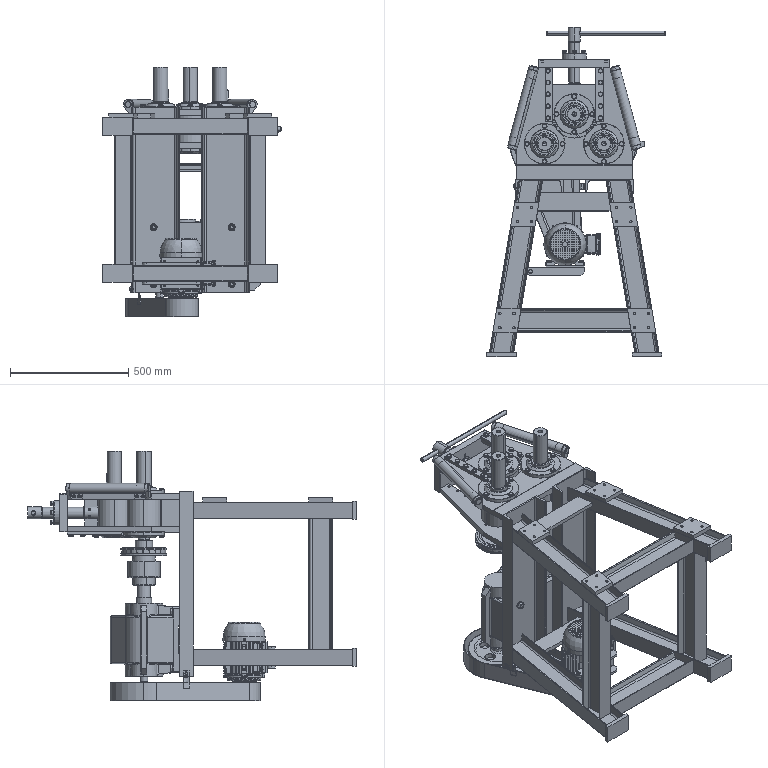Part | SolidWorks | 217 solids | 7915 faces | volume 68898357 mm3 | plane 3247 | cylinder 2250 | cone 1233 | spline 1181 | torus 4 | commonest cylinder face diameters 10 x213 16 x111 20 x106 8.376 x92 26.204 x90 10.5 x88